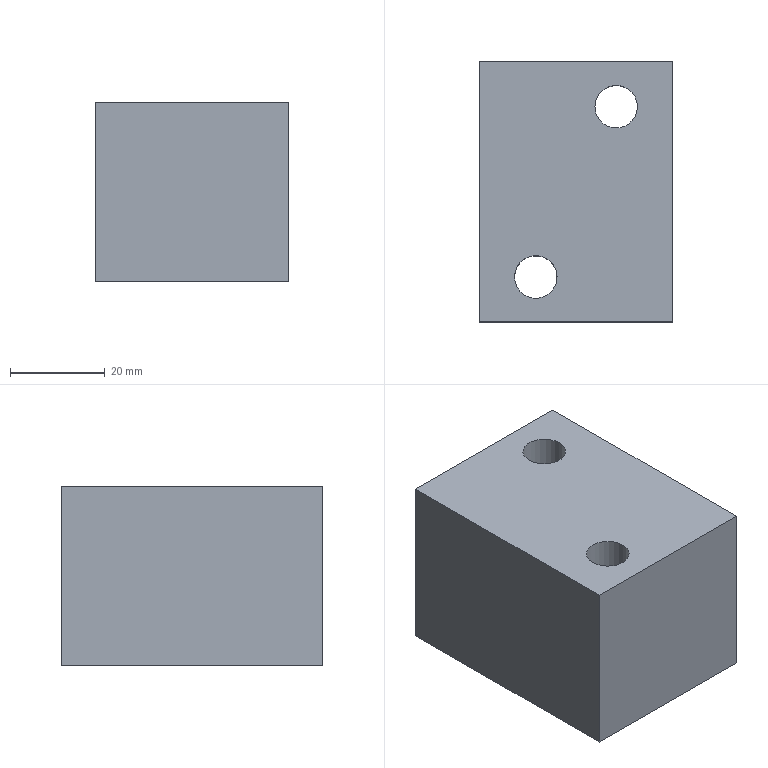Part | NX | features solid 2 | 1 solid | 12 faces | box 41 x 55 x 38 mm | volume 78205 mm3 | plane 8 | cylinder 4 | commonest cylinder face diameters 9.009 x2 14.507 x2
STEP:
#1=CARTESIAN_POINT('',(1479.246,168.,63.));
#2=VERTEX_POINT('',#1);
#3=CARTESIAN_POINT('',(1486.5,168.,63.));
#4=DIRECTION('',(0.,0.,-1.));
#5=DIRECTION('',(-1.,0.,0.));
#6=AXIS2_PLACEMENT_3D('',#3,#4,#5);
#7=CIRCLE('',#6,7.253);
#8=EDGE_CURVE('',#2,#2,#7,.F.);
#9=ORIENTED_EDGE('',*,*,#8,.T.);
#10=EDGE_LOOP('',(#9));
#11=FACE_BOUND('',#10,.T.);
#12=CARTESIAN_POINT('',(1493.754,168.,50.));
#13=VERTEX_POINT('',#12);
#14=CARTESIAN_POINT('',(1486.5,168.,50.));
#15=DIRECTION('',(0.,0.,1.));
#16=DIRECTION('',(1.,0.,0.));
#17=AXIS2_PLACEMENT_3D('',#14,#15,#16);
#18=CIRCLE('',#17,7.253);
#19=EDGE_CURVE('',#13,#13,#18,.T.);
#20=ORIENTED_EDGE('',*,*,#19,.F.);
#21=EDGE_LOOP('',(#20));
#22=FACE_BOUND('',#21,.T.);
#23=CARTESIAN_POINT('',(1486.5,168.,40.));
#24=DIRECTION('',(0.,0.,1.));
#25=DIRECTION('',(-1.,0.,0.));
#26=AXIS2_PLACEMENT_3D('',#23,#24,#25);
#27=CYLINDRICAL_SURFACE('',#26,7.253);
#28=ADVANCED_FACE('',(#11,#22),#27,.F.);
#29=CARTESIAN_POINT('',(1481.995,168.,88.));
#30=VERTEX_POINT('',#29);
#31=CARTESIAN_POINT('',(1486.5,168.,88.));
#32=DIRECTION('',(0.,0.,1.));
#33=DIRECTION('',(-1.,0.,0.));
#34=AXIS2_PLACEMENT_3D('',#31,#32,#33);
#35=CIRCLE('',#34,4.505);
#36=EDGE_CURVE('',#30,#30,#35,.F.);
#37=ORIENTED_EDGE('',*,*,#36,.F.);
#38=EDGE_LOOP('',(#37));
#39=FACE_BOUND('',#38,.T.);
#40=CARTESIAN_POINT('',(1481.995,168.,63.));
#41=VERTEX_POINT('',#40);
#42=CARTESIAN_POINT('',(1486.5,168.,63.));
#43=DIRECTION('',(0.,0.,1.));
#44=DIRECTION('',(-1.,0.,0.));
#45=AXIS2_PLACEMENT_3D('',#42,#43,#44);
#46=CIRCLE('',#45,4.505);
#47=EDGE_CURVE('',#41,#41,#46,.T.);
#48=ORIENTED_EDGE('',*,*,#47,.F.);
#49=EDGE_LOOP('',(#48));
#50=FACE_BOUND('',#49,.T.);
#51=CARTESIAN_POINT('',(1486.5,168.,35.));
#52=DIRECTION('',(0.,0.,1.));
#53=DIRECTION('',(-1.,0.,0.));
#54=AXIS2_PLACEMENT_3D('',#51,#52,#53);
#55=CYLINDRICAL_SURFACE('',#54,4.505);
#56=ADVANCED_FACE('',(#39,#50),#55,.F.);
#57=ORIENTED_EDGE('',*,*,#47,.T.);
#58=EDGE_LOOP('',(#57));
#59=FACE_BOUND('',#58,.T.);
#60=ORIENTED_EDGE('',*,*,#8,.F.);
#61=EDGE_LOOP('',(#60));
#62=FACE_BOUND('',#61,.T.);
#63=CARTESIAN_POINT('',(1486.5,193.,63.));
#64=DIRECTION('',(0.,0.,1.));
#65=DIRECTION('',(-1.,0.,0.));
#66=AXIS2_PLACEMENT_3D('',#63,#64,#65);
#67=PLANE('',#66);
#68=ADVANCED_FACE('',(#59,#62),#67,.F.);
#69=CARTESIAN_POINT('',(1474.005,132.,63.));
#70=VERTEX_POINT('',#69);
#71=CARTESIAN_POINT('',(1469.5,132.,63.));
#72=DIRECTION('',(0.,0.,1.));
#73=DIRECTION('',(1.,0.,0.));
#74=AXIS2_PLACEMENT_3D('',#71,#72,#73);
#75=CIRCLE('',#74,4.505);
#76=EDGE_CURVE('',#70,#70,#75,.T.);
#77=ORIENTED_EDGE('',*,*,#76,.T.);
#78=EDGE_LOOP('',(#77));
#79=FACE_BOUND('',#78,.T.);
#80=CARTESIAN_POINT('',(1476.754,132.,63.));
#81=VERTEX_POINT('',#80);
#82=CARTESIAN_POINT('',(1469.5,132.,63.));
#83=DIRECTION('',(0.,0.,-1.));
#84=DIRECTION('',(1.,0.,0.));
#85=AXIS2_PLACEMENT_3D('',#82,#83,#84);
#86=CIRCLE('',#85,7.253);
#87=EDGE_CURVE('',#81,#81,#86,.F.);
#88=ORIENTED_EDGE('',*,*,#87,.F.);
#89=EDGE_LOOP('',(#88));
#90=FACE_BOUND('',#89,.T.);
#91=CARTESIAN_POINT('',(1469.5,107.,63.));
#92=DIRECTION('',(0.,0.,1.));
#93=DIRECTION('',(1.,0.,0.));
#94=AXIS2_PLACEMENT_3D('',#91,#92,#93);
#95=PLANE('',#94);
#96=ADVANCED_FACE('',(#79,#90),#95,.F.);
#97=ORIENTED_EDGE('',*,*,#87,.T.);
#98=EDGE_LOOP('',(#97));
#99=FACE_BOUND('',#98,.T.);
#100=CARTESIAN_POINT('',(1476.754,132.,50.));
#101=VERTEX_POINT('',#100);
#102=CARTESIAN_POINT('',(1469.5,132.,50.));
#103=DIRECTION('',(0.,0.,1.));
#104=DIRECTION('',(1.,0.,0.));
#105=AXIS2_PLACEMENT_3D('',#102,#103,#104);
#106=CIRCLE('',#105,7.253);
#107=EDGE_CURVE('',#101,#101,#106,.T.);
#108=ORIENTED_EDGE('',*,*,#107,.F.);
#109=EDGE_LOOP('',(#108));
#110=FACE_BOUND('',#109,.T.);
#111=CARTESIAN_POINT('',(1469.5,132.,40.));
#112=DIRECTION('',(0.,0.,1.));
#113=DIRECTION('',(1.,0.,0.));
#114=AXIS2_PLACEMENT_3D('',#111,#112,#113);
#115=CYLINDRICAL_SURFACE('',#114,7.253);
#116=ADVANCED_FACE('',(#99,#110),#115,.F.);
#117=CARTESIAN_POINT('',(1474.005,132.,88.));
#118=VERTEX_POINT('',#117);
#119=CARTESIAN_POINT('',(1469.5,132.,88.));
#120=DIRECTION('',(0.,0.,1.));
#121=DIRECTION('',(1.,0.,0.));
#122=AXIS2_PLACEMENT_3D('',#119,#120,#121);
#123=CIRCLE('',#122,4.505);
#124=EDGE_CURVE('',#118,#118,#123,.T.);
#125=ORIENTED_EDGE('',*,*,#124,.T.);
#126=EDGE_LOOP('',(#125));
#127=FACE_BOUND('',#126,.T.);
#128=ORIENTED_EDGE('',*,*,#76,.F.);
#129=EDGE_LOOP('',(#128));
#130=FACE_BOUND('',#129,.T.);
#131=CARTESIAN_POINT('',(1469.5,132.,35.));
#132=DIRECTION('',(0.,0.,1.));
#133=DIRECTION('',(1.,0.,0.));
#134=AXIS2_PLACEMENT_3D('',#131,#132,#133);
#135=CYLINDRICAL_SURFACE('',#134,4.505);
#136=ADVANCED_FACE('',(#127,#130),#135,.F.);
#137=CARTESIAN_POINT('',(1457.5,122.5,50.));
#138=VERTEX_POINT('',#137);
#139=CARTESIAN_POINT('',(1457.5,122.5,88.));
#140=VERTEX_POINT('',#139);
#141=CARTESIAN_POINT('',(1457.5,122.5,31.));
#142=DIRECTION('',(0.,0.,-1.));
#143=VECTOR('',#142,1000.);
#144=LINE('',#141,#143);
#145=EDGE_CURVE('',#138,#140,#144,.F.);
#146=ORIENTED_EDGE('',*,*,#145,.T.);
#147=CARTESIAN_POINT('',(1457.5,177.5,88.));
#148=VERTEX_POINT('',#147);
#149=CARTESIAN_POINT('',(1457.5,126.,88.));
#150=DIRECTION('',(0.,1.,0.));
#151=VECTOR('',#150,1000.);
#152=LINE('',#149,#151);
#153=EDGE_CURVE('',#140,#148,#152,.T.);
#154=ORIENTED_EDGE('',*,*,#153,.T.);
#155=CARTESIAN_POINT('',(1457.5,177.5,50.));
#156=VERTEX_POINT('',#155);
#157=CARTESIAN_POINT('',(1457.5,177.5,30.));
#158=DIRECTION('',(0.,0.,-1.));
#159=VECTOR('',#158,1000.);
#160=LINE('',#157,#159);
#161=EDGE_CURVE('',#156,#148,#160,.F.);
#162=ORIENTED_EDGE('',*,*,#161,.F.);
#163=CARTESIAN_POINT('',(1457.5,126.,50.));
#164=DIRECTION('',(0.,1.,0.));
#165=VECTOR('',#164,1000.);
#166=LINE('',#163,#165);
#167=EDGE_CURVE('',#156,#138,#166,.F.);
#168=ORIENTED_EDGE('',*,*,#167,.T.);
#169=EDGE_LOOP('',(#146,#154,#162,#168));
#170=FACE_BOUND('',#169,.T.);
#171=CARTESIAN_POINT('',(1457.5,126.,31.));
#172=DIRECTION('',(-1.,0.,0.));
#173=DIRECTION('',(0.,0.,1.));
#174=AXIS2_PLACEMENT_3D('',#171,#172,#173);
#175=PLANE('',#174);
#176=ADVANCED_FACE('',(#170),#175,.T.);
#177=CARTESIAN_POINT('',(1498.5,177.5,88.));
#178=VERTEX_POINT('',#177);
#179=CARTESIAN_POINT('',(1545.165,177.5,88.));
#180=DIRECTION('',(-1.,0.,0.));
#181=VECTOR('',#180,1000.);
#182=LINE('',#179,#181);
#183=EDGE_CURVE('',#148,#178,#182,.F.);
#184=ORIENTED_EDGE('',*,*,#183,.T.);
#185=CARTESIAN_POINT('',(1498.5,177.5,50.));
#186=VERTEX_POINT('',#185);
#187=CARTESIAN_POINT('',(1498.5,177.5,31.));
#188=DIRECTION('',(0.,0.,-1.));
#189=VECTOR('',#188,1000.);
#190=LINE('',#187,#189);
#191=EDGE_CURVE('',#178,#186,#190,.T.);
#192=ORIENTED_EDGE('',*,*,#191,.T.);
#193=CARTESIAN_POINT('',(1545.165,177.5,50.));
#194=DIRECTION('',(-1.,0.,0.));
#195=VECTOR('',#194,1000.);
#196=LINE('',#193,#195);
#197=EDGE_CURVE('',#186,#156,#196,.T.);
#198=ORIENTED_EDGE('',*,*,#197,.T.);
#199=ORIENTED_EDGE('',*,*,#161,.T.);
#200=EDGE_LOOP('',(#184,#192,#198,#199));
#201=FACE_BOUND('',#200,.T.);
#202=CARTESIAN_POINT('',(1545.165,177.5,30.));
#203=DIRECTION('',(0.,-1.,0.));
#204=DIRECTION('',(0.,0.,-1.));
#205=AXIS2_PLACEMENT_3D('',#202,#203,#204);
#206=PLANE('',#205);
#207=ADVANCED_FACE('',(#201),#206,.F.);
#208=CARTESIAN_POINT('',(1498.5,122.5,50.));
#209=VERTEX_POINT('',#208);
#210=CARTESIAN_POINT('',(1498.5,122.5,88.));
#211=VERTEX_POINT('',#210);
#212=CARTESIAN_POINT('',(1498.5,122.5,31.));
#213=DIRECTION('',(0.,0.,1.));
#214=VECTOR('',#213,1000.);
#215=LINE('',#212,#214);
#216=EDGE_CURVE('',#209,#211,#215,.T.);
#217=ORIENTED_EDGE('',*,*,#216,.F.);
#218=CARTESIAN_POINT('',(1498.5,126.,50.));
#219=DIRECTION('',(0.,-1.,0.));
#220=VECTOR('',#219,1000.);
#221=LINE('',#218,#220);
#222=EDGE_CURVE('',#209,#186,#221,.F.);
#223=ORIENTED_EDGE('',*,*,#222,.T.);
#224=ORIENTED_EDGE('',*,*,#191,.F.);
#225=CARTESIAN_POINT('',(1498.5,126.,88.));
#226=DIRECTION('',(0.,-1.,0.));
#227=VECTOR('',#226,1000.);
#228=LINE('',#225,#227);
#229=EDGE_CURVE('',#178,#211,#228,.T.);
#230=ORIENTED_EDGE('',*,*,#229,.T.);
#231=EDGE_LOOP('',(#217,#223,#224,#230));
#232=FACE_BOUND('',#231,.T.);
#233=CARTESIAN_POINT('',(1498.5,126.,31.));
#234=DIRECTION('',(1.,0.,0.));
#235=DIRECTION('',(0.,0.,-1.));
#236=AXIS2_PLACEMENT_3D('',#233,#234,#235);
#237=PLANE('',#236);
#238=ADVANCED_FACE('',(#232),#237,.T.);
#239=CARTESIAN_POINT('',(1545.165,122.5,50.));
#240=DIRECTION('',(1.,0.,0.));
#241=VECTOR('',#240,1000.);
#242=LINE('',#239,#241);
#243=EDGE_CURVE('',#138,#209,#242,.T.);
#244=ORIENTED_EDGE('',*,*,#243,.T.);
#245=ORIENTED_EDGE('',*,*,#216,.T.);
#246=CARTESIAN_POINT('',(1545.165,122.5,88.));
#247=DIRECTION('',(1.,0.,0.));
#248=VECTOR('',#247,1000.);
#249=LINE('',#246,#248);
#250=EDGE_CURVE('',#211,#140,#249,.F.);
#251=ORIENTED_EDGE('',*,*,#250,.T.);
#252=ORIENTED_EDGE('',*,*,#145,.F.);
#253=EDGE_LOOP('',(#244,#245,#251,#252));
#254=FACE_BOUND('',#253,.T.);
#255=CARTESIAN_POINT('',(1545.165,122.5,30.));
#256=DIRECTION('',(0.,1.,0.));
#257=DIRECTION('',(0.,0.,1.));
#258=AXIS2_PLACEMENT_3D('',#255,#256,#257);
#259=PLANE('',#258);
#260=ADVANCED_FACE('',(#254),#259,.F.);
#261=ORIENTED_EDGE('',*,*,#36,.T.);
#262=EDGE_LOOP('',(#261));
#263=FACE_BOUND('',#262,.T.);
#264=ORIENTED_EDGE('',*,*,#250,.F.);
#265=ORIENTED_EDGE('',*,*,#229,.F.);
#266=ORIENTED_EDGE('',*,*,#183,.F.);
#267=ORIENTED_EDGE('',*,*,#153,.F.);
#268=EDGE_LOOP('',(#264,#265,#266,#267));
#269=FACE_BOUND('',#268,.T.);
#270=ORIENTED_EDGE('',*,*,#124,.F.);
#271=EDGE_LOOP('',(#270));
#272=FACE_BOUND('',#271,.T.);
#273=CARTESIAN_POINT('',(1091.879,126.,88.));
#274=DIRECTION('',(0.,0.,1.));
#275=DIRECTION('',(-1.,0.,0.));
#276=AXIS2_PLACEMENT_3D('',#273,#274,#275);
#277=PLANE('',#276);
#278=ADVANCED_FACE('',(#263,#269,#272),#277,.T.);
#279=ORIENTED_EDGE('',*,*,#19,.T.);
#280=EDGE_LOOP('',(#279));
#281=FACE_BOUND('',#280,.T.);
#282=ORIENTED_EDGE('',*,*,#222,.F.);
#283=ORIENTED_EDGE('',*,*,#243,.F.);
#284=ORIENTED_EDGE('',*,*,#167,.F.);
#285=ORIENTED_EDGE('',*,*,#197,.F.);
#286=EDGE_LOOP('',(#282,#283,#284,#285));
#287=FACE_BOUND('',#286,.T.);
#288=ORIENTED_EDGE('',*,*,#107,.T.);
#289=EDGE_LOOP('',(#288));
#290=FACE_BOUND('',#289,.T.);
#291=CARTESIAN_POINT('',(557.257,0.,50.));
#292=DIRECTION('',(0.,0.,1.));
#293=DIRECTION('',(0.,1.,0.));
#294=AXIS2_PLACEMENT_3D('',#291,#292,#293);
#295=PLANE('',#294);
#296=ADVANCED_FACE('',(#281,#287,#290),#295,.F.);
#297=CLOSED_SHELL('',(#28,#56,#68,#96,#116,#136,#176,#207,#238,#260,#278,#296));
#298=MANIFOLD_SOLID_BREP('',#297);
#299=(LENGTH_UNIT()NAMED_UNIT(*)SI_UNIT(.MILLI.,.METRE.));
#300=UNCERTAINTY_MEASURE_WITH_UNIT(LENGTH_MEASURE(0.00001),#299,'','');
#301=(NAMED_UNIT(*)PLANE_ANGLE_UNIT()SI_UNIT($,.RADIAN.));
#302=(NAMED_UNIT(*)SI_UNIT($,.STERADIAN.)SOLID_ANGLE_UNIT());
#303=(GEOMETRIC_REPRESENTATION_CONTEXT(3)GLOBAL_UNCERTAINTY_ASSIGNED_CONTEXT((#300))GLOBAL_UNIT_ASSIGNED_CONTEXT((#299,#301,#302))REPRESENTATION_CONTEXT('',''));
#304=ADVANCED_BREP_SHAPE_REPRESENTATION('',(#298),#303);